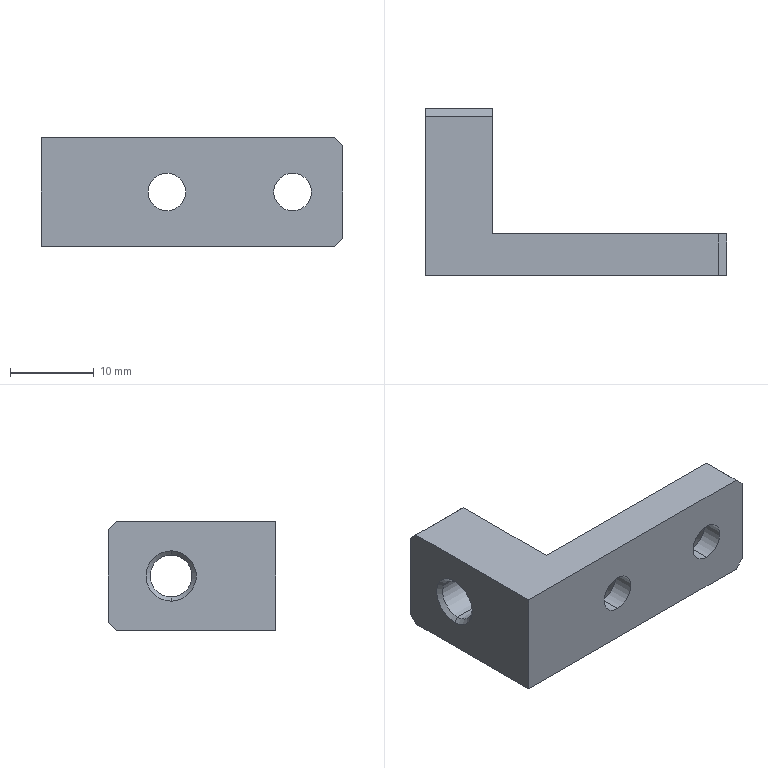Part | STEP file | PN_0074 Mount electronic clip s longitudinal manipulator limit seat | 1 solid | 26 faces | box 36 x 20 x 13 mm | volume 3451 mm3 | plane 12 | cone 8 | cylinder 6 | commonest cylinder face diameters 4.5 x4 5 x2